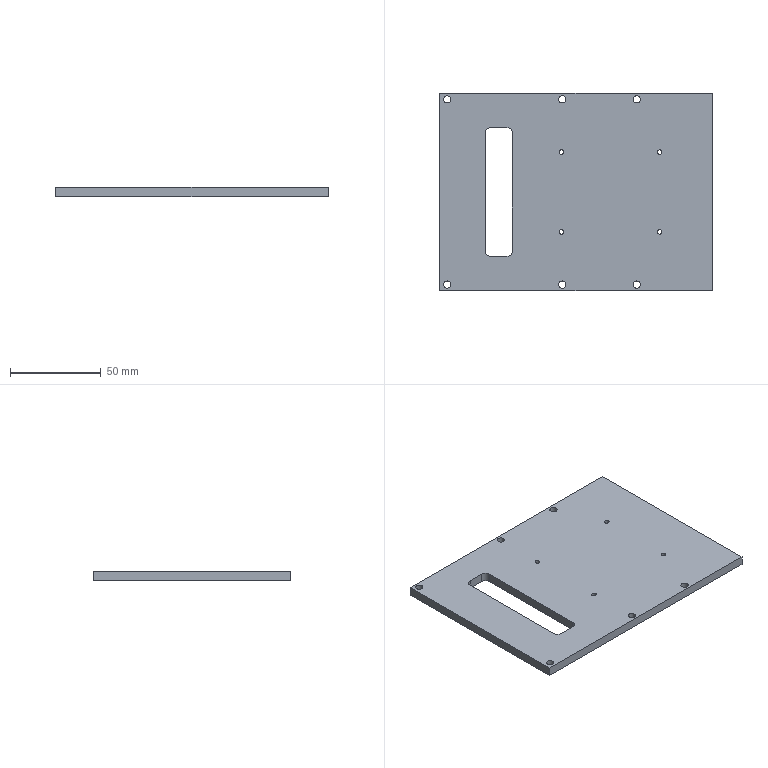CAM job | NX | 3-axis milling, drilling | part box 150 x 108.5 x 5 mm | stock box 150 x 108.5 x 5 mm
Tools:
number,name,description,diameter,corner_radius,flute_length,length,flutes
7,D6A45,Milling Tool-5 Parameters,6.0,0.0,3.0,3.0,2
12,2.5ZT,Drilling Tool,2.5,0.0,35.0,50.0,2
14,4.0ZT,Drilling Tool,4.0,0.0,35.0,50.0,2
10,D10,Milling Tool-5 Parameters,10.0,0.0,50.0,75.0,2
6,D6,Milling Tool-5 Parameters,6.0,0.0,50.0,75.0,2
13,M3,Milling Tool-5 Parameters,2.5,0.0,50.0,75.0,2
Operations:
program,operation,operation_type,tool,method,geometry_group,spindle_rpm,surface_speed,feed_per_tooth,feed_cut,feed_plunge,cut_length_mm,path_length_mm,cut_time_min,machine_time_min
1,DRILLING,Operation,D6A45,METHOD,A,3500.0,43.0,0.0357,250.0,0.0,51.5,576.92,0.206,0.2585
1,DRILLING_COPY_COPY_COPY,Operation,2.5ZT,METHOD,A,2000.0,15.0,0.03,120.0,0.0,41.004,293.296,0.3417,0.3669
1,DRILLING_COPY_COPY_COPY_COPY_1,Operation,M3,METHOD,A,200.0,1.0,0.0013,0.5,0.0,34.0,279.288,68.0,68.025
1,DRILLING_COPY_COPY_COPY_COPY,Operation,4.0ZT,METHOD,A,2000.0,15.0,0.03,120.0,0.0,64.21,514.826,0.5351,0.5801
1,ZLEVEL_PROFILE_2,ZLevelMilling,D10,METHOD,A,9500.0,298.0,0.1053,2000.0,1000.0,765.718,824.218,0.4067,0.4126
1,ZLEVEL_PROFILE_COPY_1,ZLevelMilling,D6,METHOD,A,9500.0,179.0,0.0842,1600.0,100.0,254.666,756.945,0.1592,0.2094
1,ZLEVEL_PROFILE_1,ZLevelMilling,D6,METHOD,A,9500.0,298.0,0.0526,1000.0,100.0,154.721,221.721,0.1547,0.1614
1,ZLEVEL_PROFILE_1_COPY_1_COPY_COPY_COPY_1,ZLevelMilling,D6A45,METHOD,A,9500.0,179.0,0.0526,1000.0,100.0,247.71,1709.053,0.2477,0.3938